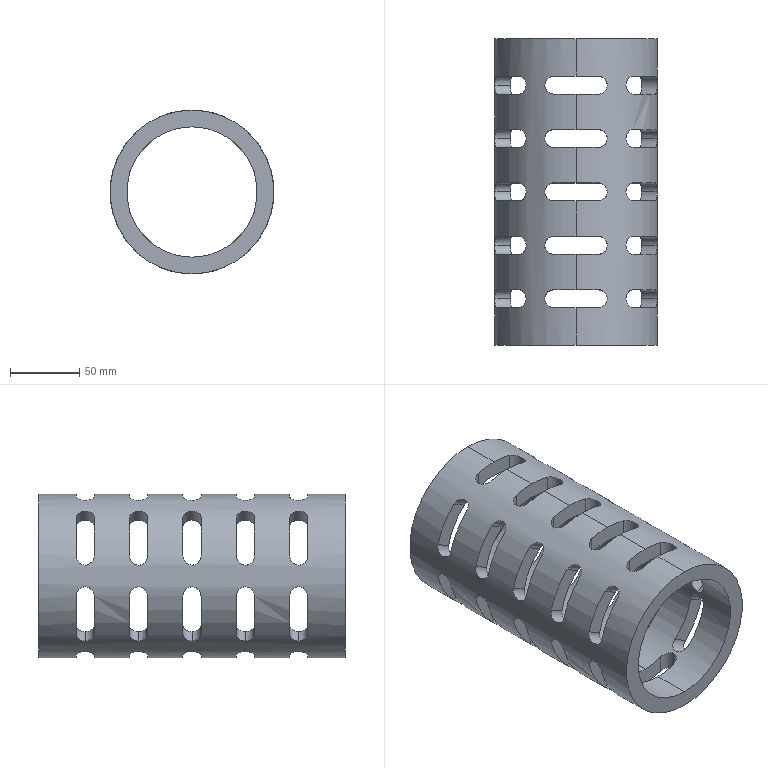Part | SolidWorks | features CirPattern 1, Extrusion 1, ICE 1, LPattern 1 | 1 solid | 161 faces | box 118 x 221 x 118 mm | volume 679782 mm3 | cylinder 99 | plane 62 | commonest cylinder face diameters 13 x95 94 x2 118 x2